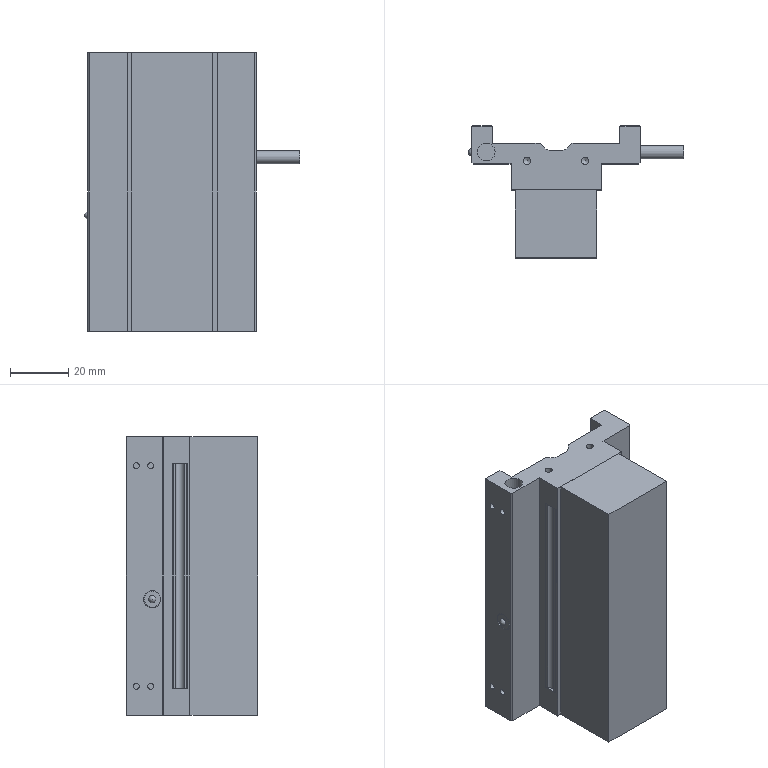Part | STEP file | BODY5_E-RAM6-S-640-ME30-C5 | 1 solid | 213 faces | box 74.25 x 45.4 x 96 mm | volume 131953 mm3 | plane 130 | cylinder 54 | cone 22 | torus 6 | sphere 1 | commonest cylinder face diameters 6 x10 2.013 x8 2.459 x6 3.242 x6 0.4 x4 2.5 x4